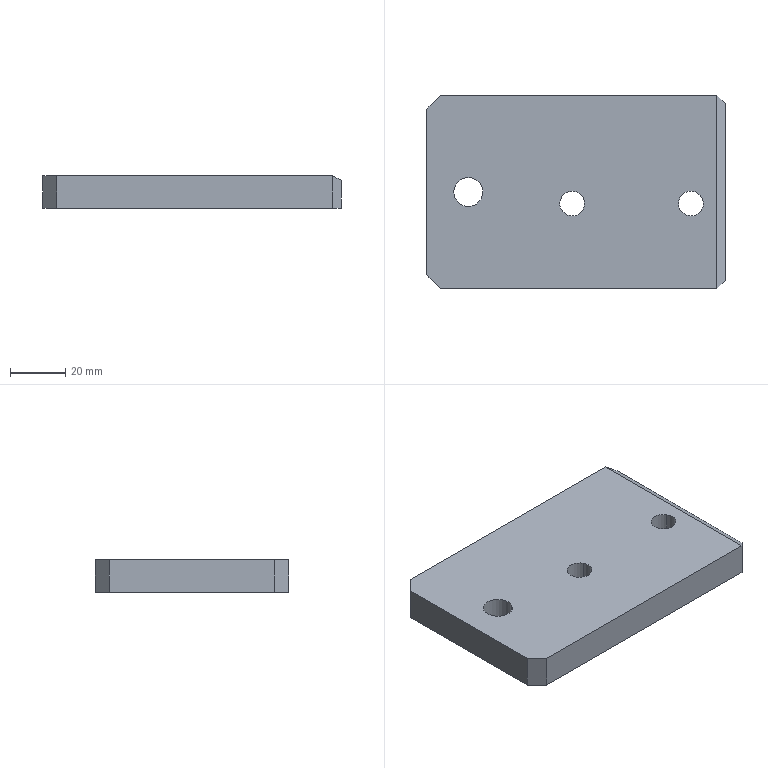Part | CATIA | 1 solid | 21 faces | box 108 x 70 x 11.8 mm | volume 85144 mm3 | plane 11 | cylinder 6 | cone 4 | commonest cylinder face diameters 9 x4 10.5 x2
STEP:
#1=CARTESIAN_POINT('',(-246.,-35.,-43.));
#2=VERTEX_POINT('',#1);
#3=CARTESIAN_POINT('',(-246.,-35.,-54.8));
#4=VERTEX_POINT('',#3);
#5=CARTESIAN_POINT('',(-246.,-35.,-48.9));
#6=DIRECTION('',(0.,0.,1.));
#7=VECTOR('',#6,1.);
#8=LINE('',#5,#7);
#9=EDGE_CURVE('',#2,#4,#8,.F.);
#10=ORIENTED_EDGE('',*,*,#9,.F.);
#11=CARTESIAN_POINT('',(-251.,-30.,-43.));
#12=VERTEX_POINT('',#11);
#13=CARTESIAN_POINT('',(-248.5,-32.5,-43.));
#14=DIRECTION('',(0.7071,-0.7071,0.));
#15=VECTOR('',#14,1.);
#16=LINE('',#13,#15);
#17=EDGE_CURVE('',#2,#12,#16,.F.);
#18=ORIENTED_EDGE('',*,*,#17,.T.);
#19=CARTESIAN_POINT('',(-251.,-30.,-54.8));
#20=VERTEX_POINT('',#19);
#21=CARTESIAN_POINT('',(-251.,-30.,-48.9));
#22=DIRECTION('',(0.,0.,1.));
#23=VECTOR('',#22,1.);
#24=LINE('',#21,#23);
#25=EDGE_CURVE('',#12,#20,#24,.F.);
#26=ORIENTED_EDGE('',*,*,#25,.T.);
#27=CARTESIAN_POINT('',(-248.5,-32.5,-54.8));
#28=DIRECTION('',(0.7071,-0.7071,0.));
#29=VECTOR('',#28,1.);
#30=LINE('',#27,#29);
#31=EDGE_CURVE('',#20,#4,#30,.T.);
#32=ORIENTED_EDGE('',*,*,#31,.T.);
#33=EDGE_LOOP('',(#10,#18,#26,#32));
#34=FACE_OUTER_BOUND('',#33,.T.);
#35=CARTESIAN_POINT('',(-251.,-30.,-57.16));
#36=DIRECTION('',(0.7071,0.7071,0.));
#37=DIRECTION('',(0.,0.,1.));
#38=AXIS2_PLACEMENT_3D('',#35,#36,#37);
#39=PLANE('',#38);
#40=ADVANCED_FACE('',(#34),#39,.F.);
#41=CARTESIAN_POINT('',(-251.,30.,-43.));
#42=VERTEX_POINT('',#41);
#43=CARTESIAN_POINT('',(-251.,30.,-54.8));
#44=VERTEX_POINT('',#43);
#45=CARTESIAN_POINT('',(-251.,30.,-48.9));
#46=DIRECTION('',(0.,0.,-1.));
#47=VECTOR('',#46,1.);
#48=LINE('',#45,#47);
#49=EDGE_CURVE('',#42,#44,#48,.T.);
#50=ORIENTED_EDGE('',*,*,#49,.T.);
#51=CARTESIAN_POINT('',(-251.,0.,-54.8));
#52=DIRECTION('',(0.,-1.,0.));
#53=VECTOR('',#52,1.);
#54=LINE('',#51,#53);
#55=EDGE_CURVE('',#44,#20,#54,.T.);
#56=ORIENTED_EDGE('',*,*,#55,.T.);
#57=ORIENTED_EDGE('',*,*,#25,.F.);
#58=CARTESIAN_POINT('',(-251.,0.,-43.));
#59=DIRECTION('',(0.,-1.,0.));
#60=VECTOR('',#59,1.);
#61=LINE('',#58,#60);
#62=EDGE_CURVE('',#42,#12,#61,.T.);
#63=ORIENTED_EDGE('',*,*,#62,.F.);
#64=EDGE_LOOP('',(#50,#56,#57,#63));
#65=FACE_OUTER_BOUND('',#64,.T.);
#66=CARTESIAN_POINT('',(-251.,35.,-43.));
#67=DIRECTION('',(1.,0.,0.));
#68=DIRECTION('',(0.,-1.,0.));
#69=AXIS2_PLACEMENT_3D('',#66,#67,#68);
#70=PLANE('',#69);
#71=ADVANCED_FACE('',(#65),#70,.F.);
#72=ORIENTED_EDGE('',*,*,#49,.F.);
#73=CARTESIAN_POINT('',(-246.,35.,-43.));
#74=VERTEX_POINT('',#73);
#75=CARTESIAN_POINT('',(-248.5,32.5,-43.));
#76=DIRECTION('',(0.7071,0.7071,0.));
#77=VECTOR('',#76,1.);
#78=LINE('',#75,#77);
#79=EDGE_CURVE('',#42,#74,#78,.T.);
#80=ORIENTED_EDGE('',*,*,#79,.T.);
#81=CARTESIAN_POINT('',(-246.,35.,-54.8));
#82=VERTEX_POINT('',#81);
#83=CARTESIAN_POINT('',(-246.,35.,-48.9));
#84=DIRECTION('',(0.,0.,-1.));
#85=VECTOR('',#84,1.);
#86=LINE('',#83,#85);
#87=EDGE_CURVE('',#74,#82,#86,.T.);
#88=ORIENTED_EDGE('',*,*,#87,.T.);
#89=CARTESIAN_POINT('',(-248.5,32.5,-54.8));
#90=DIRECTION('',(0.7071,0.7071,0.));
#91=VECTOR('',#90,1.);
#92=LINE('',#89,#91);
#93=EDGE_CURVE('',#82,#44,#92,.F.);
#94=ORIENTED_EDGE('',*,*,#93,.T.);
#95=EDGE_LOOP('',(#72,#80,#88,#94));
#96=FACE_OUTER_BOUND('',#95,.T.);
#97=CARTESIAN_POINT('',(-251.,30.,-40.64));
#98=DIRECTION('',(0.7071,-0.7071,0.));
#99=DIRECTION('',(0.,0.,-1.));
#100=AXIS2_PLACEMENT_3D('',#97,#98,#99);
#101=PLANE('',#100);
#102=ADVANCED_FACE('',(#96),#101,.F.);
#103=CARTESIAN_POINT('',(-146.,35.,-43.));
#104=VERTEX_POINT('',#103);
#105=CARTESIAN_POINT('',(-146.,35.,-54.8));
#106=VERTEX_POINT('',#105);
#107=CARTESIAN_POINT('',(-146.,35.,-48.9));
#108=DIRECTION('',(0.,0.,1.));
#109=VECTOR('',#108,1.);
#110=LINE('',#107,#109);
#111=EDGE_CURVE('',#104,#106,#110,.F.);
#112=ORIENTED_EDGE('',*,*,#111,.T.);
#113=CARTESIAN_POINT('',(-196.,35.,-54.8));
#114=DIRECTION('',(-1.,0.,0.));
#115=VECTOR('',#114,1.);
#116=LINE('',#113,#115);
#117=EDGE_CURVE('',#106,#82,#116,.T.);
#118=ORIENTED_EDGE('',*,*,#117,.T.);
#119=ORIENTED_EDGE('',*,*,#87,.F.);
#120=CARTESIAN_POINT('',(-196.,35.,-43.));
#121=DIRECTION('',(-1.,0.,0.));
#122=VECTOR('',#121,1.);
#123=LINE('',#120,#122);
#124=EDGE_CURVE('',#104,#74,#123,.T.);
#125=ORIENTED_EDGE('',*,*,#124,.F.);
#126=EDGE_LOOP('',(#112,#118,#119,#125));
#127=FACE_OUTER_BOUND('',#126,.T.);
#128=CARTESIAN_POINT('',(-143.,35.,-43.));
#129=DIRECTION('',(0.,-1.,0.));
#130=DIRECTION('',(-1.,0.,0.));
#131=AXIS2_PLACEMENT_3D('',#128,#129,#130);
#132=PLANE('',#131);
#133=ADVANCED_FACE('',(#127),#132,.F.);
#134=CARTESIAN_POINT('',(-146.,-35.,-43.));
#135=VERTEX_POINT('',#134);
#136=CARTESIAN_POINT('',(-146.,-35.,-54.8));
#137=VERTEX_POINT('',#136);
#138=CARTESIAN_POINT('',(-146.,-35.,-48.9));
#139=DIRECTION('',(0.,0.,-1.));
#140=VECTOR('',#139,1.);
#141=LINE('',#138,#140);
#142=EDGE_CURVE('',#135,#137,#141,.T.);
#143=ORIENTED_EDGE('',*,*,#142,.F.);
#144=CARTESIAN_POINT('',(-196.,-35.,-43.));
#145=DIRECTION('',(1.,0.,0.));
#146=VECTOR('',#145,1.);
#147=LINE('',#144,#146);
#148=EDGE_CURVE('',#2,#135,#147,.T.);
#149=ORIENTED_EDGE('',*,*,#148,.F.);
#150=ORIENTED_EDGE('',*,*,#9,.T.);
#151=CARTESIAN_POINT('',(-196.,-35.,-54.8));
#152=DIRECTION('',(1.,0.,0.));
#153=VECTOR('',#152,1.);
#154=LINE('',#151,#153);
#155=EDGE_CURVE('',#4,#137,#154,.T.);
#156=ORIENTED_EDGE('',*,*,#155,.T.);
#157=EDGE_LOOP('',(#143,#149,#150,#156));
#158=FACE_OUTER_BOUND('',#157,.T.);
#159=CARTESIAN_POINT('',(-251.,-35.,-43.));
#160=DIRECTION('',(0.,1.,0.));
#161=DIRECTION('',(1.,0.,0.));
#162=AXIS2_PLACEMENT_3D('',#159,#160,#161);
#163=PLANE('',#162);
#164=ADVANCED_FACE('',(#158),#163,.F.);
#165=CARTESIAN_POINT('',(-143.,32.,-44.732));
#166=VERTEX_POINT('',#165);
#167=CARTESIAN_POINT('',(-146.,35.,-43.));
#168=CARTESIAN_POINT('',(-143.,32.,-44.732));
#169=B_SPLINE_CURVE_WITH_KNOTS('',1,(#167,#168),.UNSPECIFIED.,.F.,.U.,(2,2),(-2.291,2.291),.UNSPECIFIED.);
#170=EDGE_CURVE('',#166,#104,#169,.F.);
#171=ORIENTED_EDGE('',*,*,#170,.F.);
#172=CARTESIAN_POINT('',(-143.,32.,-54.8));
#173=VERTEX_POINT('',#172);
#174=CARTESIAN_POINT('',(-143.,32.,-48.9));
#175=DIRECTION('',(0.,0.,1.));
#176=VECTOR('',#175,1.);
#177=LINE('',#174,#176);
#178=EDGE_CURVE('',#166,#173,#177,.F.);
#179=ORIENTED_EDGE('',*,*,#178,.T.);
#180=CARTESIAN_POINT('',(-144.5,33.5,-54.8));
#181=DIRECTION('',(-0.7071,0.7071,0.));
#182=VECTOR('',#181,1.);
#183=LINE('',#180,#182);
#184=EDGE_CURVE('',#173,#106,#183,.T.);
#185=ORIENTED_EDGE('',*,*,#184,.T.);
#186=ORIENTED_EDGE('',*,*,#111,.F.);
#187=EDGE_LOOP('',(#171,#179,#185,#186));
#188=FACE_OUTER_BOUND('',#187,.T.);
#189=CARTESIAN_POINT('',(-143.,32.,-57.16));
#190=DIRECTION('',(-0.7071,-0.7071,0.));
#191=DIRECTION('',(0.,0.,1.));
#192=AXIS2_PLACEMENT_3D('',#189,#190,#191);
#193=PLANE('',#192);
#194=ADVANCED_FACE('',(#188),#193,.F.);
#195=CARTESIAN_POINT('',(-143.,-32.,-44.732));
#196=VERTEX_POINT('',#195);
#197=CARTESIAN_POINT('',(-143.,0.,-44.732));
#198=DIRECTION('',(0.,-1.,0.));
#199=VECTOR('',#198,1.);
#200=LINE('',#197,#199);
#201=EDGE_CURVE('',#196,#166,#200,.F.);
#202=ORIENTED_EDGE('',*,*,#201,.F.);
#203=CARTESIAN_POINT('',(-143.,-32.,-54.8));
#204=VERTEX_POINT('',#203);
#205=CARTESIAN_POINT('',(-143.,-32.,-49.766));
#206=DIRECTION('',(0.,0.,-1.));
#207=VECTOR('',#206,1.);
#208=LINE('',#205,#207);
#209=EDGE_CURVE('',#196,#204,#208,.T.);
#210=ORIENTED_EDGE('',*,*,#209,.T.);
#211=CARTESIAN_POINT('',(-143.,0.,-54.8));
#212=DIRECTION('',(0.,1.,0.));
#213=VECTOR('',#212,1.);
#214=LINE('',#211,#213);
#215=EDGE_CURVE('',#204,#173,#214,.T.);
#216=ORIENTED_EDGE('',*,*,#215,.T.);
#217=ORIENTED_EDGE('',*,*,#178,.F.);
#218=EDGE_LOOP('',(#202,#210,#216,#217));
#219=FACE_OUTER_BOUND('',#218,.T.);
#220=CARTESIAN_POINT('',(-143.,-35.,-43.));
#221=DIRECTION('',(-1.,0.,0.));
#222=DIRECTION('',(0.,1.,0.));
#223=AXIS2_PLACEMENT_3D('',#220,#221,#222);
#224=PLANE('',#223);
#225=ADVANCED_FACE('',(#219),#224,.F.);
#226=CARTESIAN_POINT('',(-146.,-35.,-43.));
#227=CARTESIAN_POINT('',(-143.,-32.,-44.732));
#228=B_SPLINE_CURVE_WITH_KNOTS('',1,(#226,#227),.UNSPECIFIED.,.F.,.U.,(2,2),(-2.291,2.291),.UNSPECIFIED.);
#229=EDGE_CURVE('',#135,#196,#228,.T.);
#230=ORIENTED_EDGE('',*,*,#229,.F.);
#231=ORIENTED_EDGE('',*,*,#142,.T.);
#232=CARTESIAN_POINT('',(-144.5,-33.5,-54.8));
#233=DIRECTION('',(-0.7071,-0.7071,0.));
#234=VECTOR('',#233,1.);
#235=LINE('',#232,#234);
#236=EDGE_CURVE('',#137,#204,#235,.F.);
#237=ORIENTED_EDGE('',*,*,#236,.T.);
#238=ORIENTED_EDGE('',*,*,#209,.F.);
#239=EDGE_LOOP('',(#230,#231,#237,#238));
#240=FACE_OUTER_BOUND('',#239,.T.);
#241=CARTESIAN_POINT('',(-143.,-32.,-40.64));
#242=DIRECTION('',(-0.7071,0.7071,0.));
#243=DIRECTION('',(0.,0.,-1.));
#244=AXIS2_PLACEMENT_3D('',#241,#242,#243);
#245=PLANE('',#244);
#246=ADVANCED_FACE('',(#240),#245,.F.);
#247=ORIENTED_EDGE('',*,*,#170,.T.);
#248=CARTESIAN_POINT('',(-146.,0.,-43.));
#249=DIRECTION('',(0.,-1.,0.));
#250=VECTOR('',#249,1.);
#251=LINE('',#248,#250);
#252=EDGE_CURVE('',#135,#104,#251,.F.);
#253=ORIENTED_EDGE('',*,*,#252,.F.);
#254=ORIENTED_EDGE('',*,*,#229,.T.);
#255=ORIENTED_EDGE('',*,*,#201,.T.);
#256=EDGE_LOOP('',(#247,#253,#254,#255));
#257=FACE_OUTER_BOUND('',#256,.T.);
#258=CARTESIAN_POINT('',(-146.,49.,-43.));
#259=DIRECTION('',(0.5,0.,0.866));
#260=DIRECTION('',(0.,-1.,0.));
#261=AXIS2_PLACEMENT_3D('',#258,#259,#260);
#262=PLANE('',#261);
#263=ADVANCED_FACE('',(#257),#262,.T.);
#264=CARTESIAN_POINT('',(-159.349,-6.354,-43.));
#265=VERTEX_POINT('',#264);
#266=CARTESIAN_POINT('',(-151.451,-2.039,-43.));
#267=VERTEX_POINT('',#266);
#268=CARTESIAN_POINT('',(-155.4,-4.196,-43.));
#269=DIRECTION('',(0.,0.,1.));
#270=AXIS2_PLACEMENT_3D('',#268,#269,$);
#271=CIRCLE('',#270,4.5);
#272=EDGE_CURVE('',#265,#267,#271,.T.);
#273=ORIENTED_EDGE('',*,*,#272,.T.);
#274=CARTESIAN_POINT('',(-151.451,-2.039,-49.8));
#275=VERTEX_POINT('',#274);
#276=CARTESIAN_POINT('',(-151.451,-2.039,-46.2));
#277=DIRECTION('',(0.,0.,1.));
#278=VECTOR('',#277,1.);
#279=LINE('',#276,#278);
#280=EDGE_CURVE('',#267,#275,#279,.F.);
#281=ORIENTED_EDGE('',*,*,#280,.T.);
#282=CARTESIAN_POINT('',(-159.349,-6.354,-49.8));
#283=VERTEX_POINT('',#282);
#284=CARTESIAN_POINT('',(-155.4,-4.196,-49.8));
#285=DIRECTION('',(0.,0.,1.));
#286=AXIS2_PLACEMENT_3D('',#284,#285,$);
#287=CIRCLE('',#286,4.5);
#288=EDGE_CURVE('',#283,#275,#287,.T.);
#289=ORIENTED_EDGE('',*,*,#288,.F.);
#290=CARTESIAN_POINT('',(-159.349,-6.354,-46.2));
#291=DIRECTION('',(0.,0.,1.));
#292=VECTOR('',#291,1.);
#293=LINE('',#290,#292);
#294=EDGE_CURVE('',#265,#283,#293,.F.);
#295=ORIENTED_EDGE('',*,*,#294,.F.);
#296=EDGE_LOOP('',(#273,#281,#289,#295));
#297=FACE_OUTER_BOUND('',#296,.T.);
#298=CARTESIAN_POINT('',(-155.4,-4.196,-54.7));
#299=DIRECTION('',(0.,0.,1.));
#300=DIRECTION('',(0.8776,0.4794,0.));
#301=AXIS2_PLACEMENT_3D('',#298,#299,#300);
#302=CYLINDRICAL_SURFACE('',#301,4.5);
#303=ADVANCED_FACE('',(#297),#302,.F.);
#304=CARTESIAN_POINT('',(-155.4,-4.196,-43.));
#305=DIRECTION('',(0.,0.,1.));
#306=AXIS2_PLACEMENT_3D('',#304,#305,$);
#307=CIRCLE('',#306,4.5);
#308=EDGE_CURVE('',#267,#265,#307,.T.);
#309=ORIENTED_EDGE('',*,*,#308,.T.);
#310=ORIENTED_EDGE('',*,*,#294,.T.);
#311=CARTESIAN_POINT('',(-155.4,-4.196,-49.8));
#312=DIRECTION('',(0.,0.,1.));
#313=AXIS2_PLACEMENT_3D('',#311,#312,$);
#314=CIRCLE('',#313,4.5);
#315=EDGE_CURVE('',#275,#283,#314,.T.);
#316=ORIENTED_EDGE('',*,*,#315,.F.);
#317=ORIENTED_EDGE('',*,*,#280,.F.);
#318=EDGE_LOOP('',(#309,#310,#316,#317));
#319=FACE_OUTER_BOUND('',#318,.T.);
#320=ADVANCED_FACE('',(#319),#302,.F.);
#321=CARTESIAN_POINT('',(-163.737,-8.751,-54.8));
#322=VERTEX_POINT('',#321);
#323=CARTESIAN_POINT('',(-147.063,0.3584,-54.8));
#324=VERTEX_POINT('',#323);
#325=CARTESIAN_POINT('',(-155.4,-4.196,-54.8));
#326=DIRECTION('',(0.,0.,-1.));
#327=AXIS2_PLACEMENT_3D('',#325,#326,$);
#328=CIRCLE('',#327,9.5);
#329=EDGE_CURVE('',#322,#324,#328,.F.);
#330=ORIENTED_EDGE('',*,*,#329,.F.);
#331=CARTESIAN_POINT('',(-161.693,-7.634,-52.471));
#332=DIRECTION('',(-0.6205,-0.339,-0.7071));
#333=VECTOR('',#332,1.);
#334=LINE('',#331,#333);
#335=EDGE_CURVE('',#283,#322,#334,.T.);
#336=ORIENTED_EDGE('',*,*,#335,.F.);
#337=ORIENTED_EDGE('',*,*,#288,.T.);
#338=CARTESIAN_POINT('',(-149.107,-0.7584,-52.471));
#339=DIRECTION('',(0.6205,0.339,-0.7071));
#340=VECTOR('',#339,1.);
#341=LINE('',#338,#340);
#342=EDGE_CURVE('',#275,#324,#341,.T.);
#343=ORIENTED_EDGE('',*,*,#342,.T.);
#344=EDGE_LOOP('',(#330,#336,#337,#343));
#345=FACE_OUTER_BOUND('',#344,.T.);
#346=CARTESIAN_POINT('',(-155.4,-4.196,-49.8));
#347=DIRECTION('',(0.,0.,-1.));
#348=DIRECTION('',(0.8776,0.4794,0.));
#349=AXIS2_PLACEMENT_3D('',#346,#347,#348);
#350=CONICAL_SURFACE('',#349,4.5,0.7854);
#351=ADVANCED_FACE('',(#345),#350,.F.);
#352=CARTESIAN_POINT('',(-155.4,-4.196,-54.8));
#353=DIRECTION('',(0.,0.,-1.));
#354=AXIS2_PLACEMENT_3D('',#352,#353,$);
#355=CIRCLE('',#354,9.5);
#356=EDGE_CURVE('',#324,#322,#355,.F.);
#357=ORIENTED_EDGE('',*,*,#356,.F.);
#358=ORIENTED_EDGE('',*,*,#342,.F.);
#359=ORIENTED_EDGE('',*,*,#315,.T.);
#360=ORIENTED_EDGE('',*,*,#335,.T.);
#361=EDGE_LOOP('',(#357,#358,#359,#360));
#362=FACE_OUTER_BOUND('',#361,.T.);
#363=ADVANCED_FACE('',(#362),#350,.F.);
#364=CARTESIAN_POINT('',(-202.349,-6.354,-43.));
#365=VERTEX_POINT('',#364);
#366=CARTESIAN_POINT('',(-194.451,-2.039,-43.));
#367=VERTEX_POINT('',#366);
#368=CARTESIAN_POINT('',(-198.4,-4.196,-43.));
#369=DIRECTION('',(0.,0.,1.));
#370=AXIS2_PLACEMENT_3D('',#368,#369,$);
#371=CIRCLE('',#370,4.5);
#372=EDGE_CURVE('',#365,#367,#371,.T.);
#373=ORIENTED_EDGE('',*,*,#372,.T.);
#374=CARTESIAN_POINT('',(-194.451,-2.039,-49.8));
#375=VERTEX_POINT('',#374);
#376=CARTESIAN_POINT('',(-194.451,-2.039,-46.2));
#377=DIRECTION('',(0.,0.,1.));
#378=VECTOR('',#377,1.);
#379=LINE('',#376,#378);
#380=EDGE_CURVE('',#367,#375,#379,.F.);
#381=ORIENTED_EDGE('',*,*,#380,.T.);
#382=CARTESIAN_POINT('',(-202.349,-6.354,-49.8));
#383=VERTEX_POINT('',#382);
#384=CARTESIAN_POINT('',(-198.4,-4.196,-49.8));
#385=DIRECTION('',(0.,0.,1.));
#386=AXIS2_PLACEMENT_3D('',#384,#385,$);
#387=CIRCLE('',#386,4.5);
#388=EDGE_CURVE('',#383,#375,#387,.T.);
#389=ORIENTED_EDGE('',*,*,#388,.F.);
#390=CARTESIAN_POINT('',(-202.349,-6.354,-46.2));
#391=DIRECTION('',(0.,0.,1.));
#392=VECTOR('',#391,1.);
#393=LINE('',#390,#392);
#394=EDGE_CURVE('',#365,#383,#393,.F.);
#395=ORIENTED_EDGE('',*,*,#394,.F.);
#396=EDGE_LOOP('',(#373,#381,#389,#395));
#397=FACE_OUTER_BOUND('',#396,.T.);
#398=CARTESIAN_POINT('',(-198.4,-4.196,-54.7));
#399=DIRECTION('',(0.,0.,1.));
#400=DIRECTION('',(0.8776,0.4794,0.));
#401=AXIS2_PLACEMENT_3D('',#398,#399,#400);
#402=CYLINDRICAL_SURFACE('',#401,4.5);
#403=ADVANCED_FACE('',(#397),#402,.F.);
#404=CARTESIAN_POINT('',(-198.4,-4.196,-43.));
#405=DIRECTION('',(0.,0.,1.));
#406=AXIS2_PLACEMENT_3D('',#404,#405,$);
#407=CIRCLE('',#406,4.5);
#408=EDGE_CURVE('',#367,#365,#407,.T.);
#409=ORIENTED_EDGE('',*,*,#408,.T.);
#410=ORIENTED_EDGE('',*,*,#394,.T.);
#411=CARTESIAN_POINT('',(-198.4,-4.196,-49.8));
#412=DIRECTION('',(0.,0.,1.));
#413=AXIS2_PLACEMENT_3D('',#411,#412,$);
#414=CIRCLE('',#413,4.5);
#415=EDGE_CURVE('',#375,#383,#414,.T.);
#416=ORIENTED_EDGE('',*,*,#415,.F.);
#417=ORIENTED_EDGE('',*,*,#380,.F.);
#418=EDGE_LOOP('',(#409,#410,#416,#417));
#419=FACE_OUTER_BOUND('',#418,.T.);
#420=ADVANCED_FACE('',(#419),#402,.F.);
#421=CARTESIAN_POINT('',(-206.737,-8.751,-54.8));
#422=VERTEX_POINT('',#421);
#423=CARTESIAN_POINT('',(-190.063,0.3584,-54.8));
#424=VERTEX_POINT('',#423);
#425=CARTESIAN_POINT('',(-198.4,-4.196,-54.8));
#426=DIRECTION('',(0.,0.,-1.));
#427=AXIS2_PLACEMENT_3D('',#425,#426,$);
#428=CIRCLE('',#427,9.5);
#429=EDGE_CURVE('',#422,#424,#428,.F.);
#430=ORIENTED_EDGE('',*,*,#429,.F.);
#431=CARTESIAN_POINT('',(-204.693,-7.634,-52.471));
#432=DIRECTION('',(-0.6205,-0.339,-0.7071));
#433=VECTOR('',#432,1.);
#434=LINE('',#431,#433);
#435=EDGE_CURVE('',#383,#422,#434,.T.);
#436=ORIENTED_EDGE('',*,*,#435,.F.);
#437=ORIENTED_EDGE('',*,*,#388,.T.);
#438=CARTESIAN_POINT('',(-192.107,-0.7584,-52.471));
#439=DIRECTION('',(0.6205,0.339,-0.7071));
#440=VECTOR('',#439,1.);
#441=LINE('',#438,#440);
#442=EDGE_CURVE('',#375,#424,#441,.T.);
#443=ORIENTED_EDGE('',*,*,#442,.T.);
#444=EDGE_LOOP('',(#430,#436,#437,#443));
#445=FACE_OUTER_BOUND('',#444,.T.);
#446=CARTESIAN_POINT('',(-198.4,-4.196,-49.8));
#447=DIRECTION('',(0.,0.,-1.));
#448=DIRECTION('',(0.8776,0.4794,0.));
#449=AXIS2_PLACEMENT_3D('',#446,#447,#448);
#450=CONICAL_SURFACE('',#449,4.5,0.7854);
#451=ADVANCED_FACE('',(#445),#450,.F.);
#452=CARTESIAN_POINT('',(-198.4,-4.196,-54.8));
#453=DIRECTION('',(0.,0.,-1.));
#454=AXIS2_PLACEMENT_3D('',#452,#453,$);
#455=CIRCLE('',#454,9.5);
#456=EDGE_CURVE('',#424,#422,#455,.F.);
#457=ORIENTED_EDGE('',*,*,#456,.F.);
#458=ORIENTED_EDGE('',*,*,#442,.F.);
#459=ORIENTED_EDGE('',*,*,#415,.T.);
#460=ORIENTED_EDGE('',*,*,#435,.T.);
#461=EDGE_LOOP('',(#457,#458,#459,#460));
#462=FACE_OUTER_BOUND('',#461,.T.);
#463=ADVANCED_FACE('',(#462),#450,.F.);
#464=ORIENTED_EDGE('',*,*,#236,.F.);
#465=ORIENTED_EDGE('',*,*,#155,.F.);
#466=ORIENTED_EDGE('',*,*,#31,.F.);
#467=ORIENTED_EDGE('',*,*,#55,.F.);
#468=ORIENTED_EDGE('',*,*,#93,.F.);
#469=ORIENTED_EDGE('',*,*,#117,.F.);
#470=ORIENTED_EDGE('',*,*,#184,.F.);
#471=ORIENTED_EDGE('',*,*,#215,.F.);
#472=EDGE_LOOP('',(#464,#465,#466,#467,#468,#469,#470,#471));
#473=FACE_OUTER_BOUND('',#472,.T.);
#474=CARTESIAN_POINT('',(-231.393,-2.517,-54.8));
#475=VERTEX_POINT('',#474);
#476=CARTESIAN_POINT('',(-240.607,2.517,-54.8));
#477=VERTEX_POINT('',#476);
#478=CARTESIAN_POINT('',(-236.,0.,-54.8));
#479=DIRECTION('',(0.,0.,1.));
#480=AXIS2_PLACEMENT_3D('',#478,#479,$);
#481=CIRCLE('',#480,5.25);
#482=EDGE_CURVE('',#475,#477,#481,.T.);
#483=ORIENTED_EDGE('',*,*,#482,.T.);
#484=CARTESIAN_POINT('',(-236.,0.,-54.8));
#485=DIRECTION('',(0.,0.,1.));
#486=AXIS2_PLACEMENT_3D('',#484,#485,$);
#487=CIRCLE('',#486,5.25);
#488=EDGE_CURVE('',#477,#475,#487,.T.);
#489=ORIENTED_EDGE('',*,*,#488,.T.);
#490=EDGE_LOOP('',(#483,#489));
#491=FACE_BOUND('',#490,.T.);
#492=ORIENTED_EDGE('',*,*,#456,.T.);
#493=ORIENTED_EDGE('',*,*,#429,.T.);
#494=EDGE_LOOP('',(#492,#493));
#495=FACE_BOUND('',#494,.T.);
#496=ORIENTED_EDGE('',*,*,#356,.T.);
#497=ORIENTED_EDGE('',*,*,#329,.T.);
#498=EDGE_LOOP('',(#496,#497));
#499=FACE_BOUND('',#498,.T.);
#500=CARTESIAN_POINT('',(0.,0.,-54.8));
#501=DIRECTION('',(0.,0.,1.));
#502=DIRECTION('',(1.,0.,0.));
#503=AXIS2_PLACEMENT_3D('',#500,#501,#502);
#504=PLANE('',#503);
#505=ADVANCED_FACE('',(#473,#491,#495,#499),#504,.F.);
#506=ORIENTED_EDGE('',*,*,#124,.T.);
#507=ORIENTED_EDGE('',*,*,#79,.F.);
#508=ORIENTED_EDGE('',*,*,#62,.T.);
#509=ORIENTED_EDGE('',*,*,#17,.F.);
#510=ORIENTED_EDGE('',*,*,#148,.T.);
#511=ORIENTED_EDGE('',*,*,#252,.T.);
#512=EDGE_LOOP('',(#506,#507,#508,#509,#510,#511));
#513=FACE_OUTER_BOUND('',#512,.T.);
#514=CARTESIAN_POINT('',(-231.393,-2.517,-43.));
#515=VERTEX_POINT('',#514);
#516=CARTESIAN_POINT('',(-240.607,2.517,-43.));
#517=VERTEX_POINT('',#516);
#518=CARTESIAN_POINT('',(-236.,0.,-43.));
#519=DIRECTION('',(0.,0.,1.));
#520=AXIS2_PLACEMENT_3D('',#518,#519,$);
#521=CIRCLE('',#520,5.25);
#522=EDGE_CURVE('',#515,#517,#521,.T.);
#523=ORIENTED_EDGE('',*,*,#522,.F.);
#524=CARTESIAN_POINT('',(-236.,0.,-43.));
#525=DIRECTION('',(0.,0.,1.));
#526=AXIS2_PLACEMENT_3D('',#524,#525,$);
#527=CIRCLE('',#526,5.25);
#528=EDGE_CURVE('',#517,#515,#527,.T.);
#529=ORIENTED_EDGE('',*,*,#528,.F.);
#530=EDGE_LOOP('',(#523,#529));
#531=FACE_BOUND('',#530,.T.);
#532=ORIENTED_EDGE('',*,*,#372,.F.);
#533=ORIENTED_EDGE('',*,*,#408,.F.);
#534=EDGE_LOOP('',(#532,#533));
#535=FACE_BOUND('',#534,.T.);
#536=ORIENTED_EDGE('',*,*,#272,.F.);
#537=ORIENTED_EDGE('',*,*,#308,.F.);
#538=EDGE_LOOP('',(#536,#537));
#539=FACE_BOUND('',#538,.T.);
#540=CARTESIAN_POINT('',(0.,0.,-43.));
#541=DIRECTION('',(0.,0.,1.));
#542=DIRECTION('',(1.,0.,0.));
#543=AXIS2_PLACEMENT_3D('',#540,#541,#542);
#544=PLANE('',#543);
#545=ADVANCED_FACE('',(#513,#531,#535,#539),#544,.T.);
#546=ORIENTED_EDGE('',*,*,#482,.F.);
#547=CARTESIAN_POINT('',(-231.393,-2.517,-52.8));
#548=DIRECTION('',(0.,0.,-1.));
#549=VECTOR('',#548,1.);
#550=LINE('',#547,#549);
#551=EDGE_CURVE('',#475,#515,#550,.F.);
#552=ORIENTED_EDGE('',*,*,#551,.T.);
#553=ORIENTED_EDGE('',*,*,#522,.T.);
#554=CARTESIAN_POINT('',(-240.607,2.517,-52.8));
#555=DIRECTION('',(0.,0.,-1.));
#556=VECTOR('',#555,1.);
#557=LINE('',#554,#556);
#558=EDGE_CURVE('',#477,#517,#557,.F.);
#559=ORIENTED_EDGE('',*,*,#558,.F.);
#560=EDGE_LOOP('',(#546,#552,#553,#559));
#561=FACE_OUTER_BOUND('',#560,.T.);
#562=CARTESIAN_POINT('',(-236.,0.,-43.1));
#563=DIRECTION('',(0.,0.,-1.));
#564=DIRECTION('',(0.8776,-0.4794,0.));
#565=AXIS2_PLACEMENT_3D('',#562,#563,#564);
#566=CYLINDRICAL_SURFACE('',#565,5.25);
#567=ADVANCED_FACE('',(#561),#566,.F.);
#568=ORIENTED_EDGE('',*,*,#488,.F.);
#569=ORIENTED_EDGE('',*,*,#558,.T.);
#570=ORIENTED_EDGE('',*,*,#528,.T.);
#571=ORIENTED_EDGE('',*,*,#551,.F.);
#572=EDGE_LOOP('',(#568,#569,#570,#571));
#573=FACE_OUTER_BOUND('',#572,.T.);
#574=ADVANCED_FACE('',(#573),#566,.F.);
#575=CLOSED_SHELL('',(#40,#71,#102,#133,#164,#194,#225,#246,#263,#303,#320,#351,#363,#403,#420,#451,#463,#505,#545,#567,#574));
#576=MANIFOLD_SOLID_BREP('',#575);
#577=(LENGTH_UNIT()NAMED_UNIT(*)SI_UNIT(.MILLI.,.METRE.));
#578=UNCERTAINTY_MEASURE_WITH_UNIT(LENGTH_MEASURE(0.005),#577,'','');
#579=(NAMED_UNIT(*)PLANE_ANGLE_UNIT()SI_UNIT($,.RADIAN.));
#580=(NAMED_UNIT(*)SI_UNIT($,.STERADIAN.)SOLID_ANGLE_UNIT());
#581=(GEOMETRIC_REPRESENTATION_CONTEXT(3)GLOBAL_UNCERTAINTY_ASSIGNED_CONTEXT((#578))GLOBAL_UNIT_ASSIGNED_CONTEXT((#577,#579,#580))REPRESENTATION_CONTEXT('',''));
#582=ADVANCED_BREP_SHAPE_REPRESENTATION('',(#576),#581);